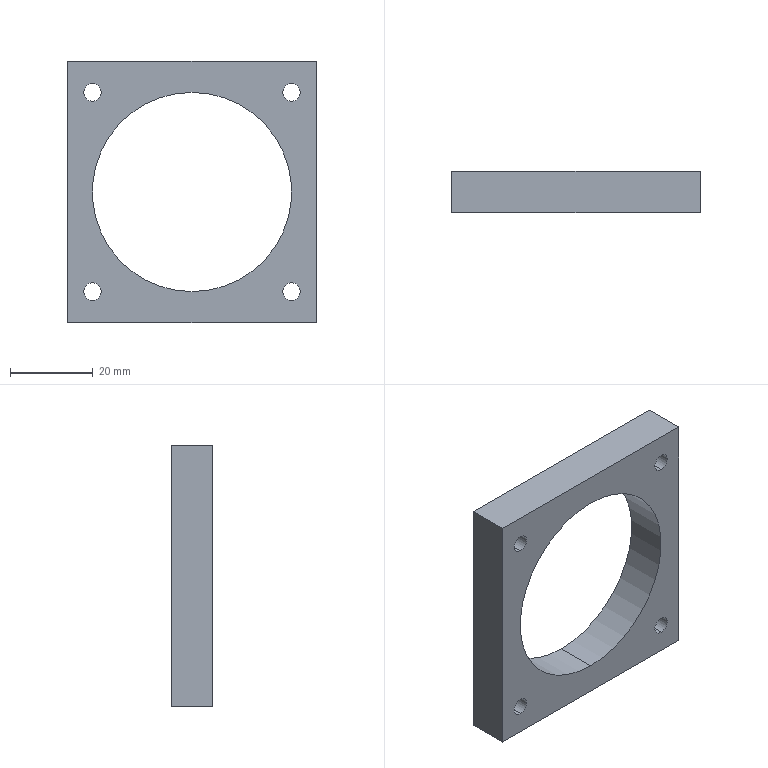Part | STEP file | 连接Plate 3 | 1 solid | 16 faces | box 60 x 10 x 63 mm | volume 19150 mm3 | cylinder 10 | plane 6 | commonest cylinder face diameters 4.2 x8 48 x2
STEP:
#1=CARTESIAN_POINT('',(0.,0.,0.));
#2=DIRECTION('',(0.,0.,1.));
#3=DIRECTION('',(1.,0.,0.));
#4=AXIS2_PLACEMENT_3D('',#1,#2,#3);
#5=CARTESIAN_POINT('',(24.,10.,21.9));
#6=VERTEX_POINT('',#5);
#7=CARTESIAN_POINT('',(24.,0.,21.9));
#8=VERTEX_POINT('',#7);
#9=CARTESIAN_POINT('',(24.,0.,21.9));
#10=DIRECTION('',(0.,-1.,0.));
#11=VECTOR('',#10,1.);
#12=LINE('',#9,#11);
#13=CARTESIAN_POINT('',(24.,0.,24.));
#14=DIRECTION('',(0.,-1.,0.));
#15=DIRECTION('',(0.,0.,-1.));
#16=AXIS2_PLACEMENT_3D('',#13,#14,#15);
#17=CYLINDRICAL_SURFACE('',#16,2.1);
#18=CARTESIAN_POINT('',(6.283,0.));
#19=DIRECTION('',(0.,1.));
#20=VECTOR('',#19,1.);
#21=LINE('',#18,#20);
#22=(GEOMETRIC_REPRESENTATION_CONTEXT(2)PARAMETRIC_REPRESENTATION_CONTEXT()REPRESENTATION_CONTEXT('',''));
#23=DEFINITIONAL_REPRESENTATION('',(#21),#22);
#24=PCURVE('',#17,#23);
#25=CARTESIAN_POINT('',(24.,0.,24.));
#26=DIRECTION('',(0.,-1.,0.));
#27=DIRECTION('',(0.,0.,-1.));
#28=AXIS2_PLACEMENT_3D('',#25,#26,#27);
#29=CYLINDRICAL_SURFACE('',#28,2.1);
#30=CARTESIAN_POINT('',(0.,0.));
#31=DIRECTION('',(0.,1.));
#32=VECTOR('',#31,1.);
#33=LINE('',#30,#32);
#34=(GEOMETRIC_REPRESENTATION_CONTEXT(2)PARAMETRIC_REPRESENTATION_CONTEXT()REPRESENTATION_CONTEXT('',''));
#35=DEFINITIONAL_REPRESENTATION('',(#33),#34);
#36=PCURVE('',#29,#35);
#37=SURFACE_CURVE('',#12,(#24,#36),.PCURVE_S1.);
#38=EDGE_CURVE('',#6,#8,#37,.T.);
#39=ORIENTED_EDGE('',*,*,#38,.T.);
#40=CARTESIAN_POINT('',(24.,0.,26.1));
#41=VERTEX_POINT('',#40);
#42=CARTESIAN_POINT('',(24.,0.,24.));
#43=DIRECTION('',(0.,-1.,0.));
#44=DIRECTION('',(0.,0.,-1.));
#45=AXIS2_PLACEMENT_3D('',#42,#43,#44);
#46=CIRCLE('',#45,2.1);
#47=CARTESIAN_POINT('',(0.,0.));
#48=DIRECTION('',(1.,0.));
#49=VECTOR('',#48,1.);
#50=LINE('',#47,#49);
#51=(GEOMETRIC_REPRESENTATION_CONTEXT(2)PARAMETRIC_REPRESENTATION_CONTEXT()REPRESENTATION_CONTEXT('',''));
#52=DEFINITIONAL_REPRESENTATION('',(#50),#51);
#53=PCURVE('',#17,#52);
#54=CARTESIAN_POINT('',(0.,0.,0.));
#55=DIRECTION('',(0.,-1.,0.));
#56=DIRECTION('',(0.,0.,-1.));
#57=AXIS2_PLACEMENT_3D('',#54,#55,#56);
#58=PLANE('',#57);
#59=CARTESIAN_POINT('',(-24.,24.));
#60=DIRECTION('',(1.,0.));
#61=AXIS2_PLACEMENT_2D('',#59,#60);
#62=CIRCLE('',#61,2.1);
#63=(GEOMETRIC_REPRESENTATION_CONTEXT(2)PARAMETRIC_REPRESENTATION_CONTEXT()REPRESENTATION_CONTEXT('',''));
#64=DEFINITIONAL_REPRESENTATION('',(#62),#63);
#65=PCURVE('',#58,#64);
#66=SURFACE_CURVE('',#46,(#53,#65),.PCURVE_S1.);
#67=EDGE_CURVE('',#41,#8,#66,.T.);
#68=ORIENTED_EDGE('',*,*,#67,.F.);
#69=CARTESIAN_POINT('',(24.,10.,26.1));
#70=VERTEX_POINT('',#69);
#71=CARTESIAN_POINT('',(24.,0.,26.1));
#72=DIRECTION('',(0.,-1.,0.));
#73=VECTOR('',#72,1.);
#74=LINE('',#71,#73);
#75=CARTESIAN_POINT('',(3.142,0.));
#76=DIRECTION('',(0.,1.));
#77=VECTOR('',#76,1.);
#78=LINE('',#75,#77);
#79=(GEOMETRIC_REPRESENTATION_CONTEXT(2)PARAMETRIC_REPRESENTATION_CONTEXT()REPRESENTATION_CONTEXT('',''));
#80=DEFINITIONAL_REPRESENTATION('',(#78),#79);
#81=PCURVE('',#17,#80);
#82=CARTESIAN_POINT('',(3.142,0.));
#83=DIRECTION('',(0.,1.));
#84=VECTOR('',#83,1.);
#85=LINE('',#82,#84);
#86=(GEOMETRIC_REPRESENTATION_CONTEXT(2)PARAMETRIC_REPRESENTATION_CONTEXT()REPRESENTATION_CONTEXT('',''));
#87=DEFINITIONAL_REPRESENTATION('',(#85),#86);
#88=PCURVE('',#29,#87);
#89=SURFACE_CURVE('',#74,(#81,#88),.PCURVE_S1.);
#90=EDGE_CURVE('',#70,#41,#89,.T.);
#91=ORIENTED_EDGE('',*,*,#90,.F.);
#92=CARTESIAN_POINT('',(24.,10.,24.));
#93=DIRECTION('',(0.,-1.,0.));
#94=DIRECTION('',(0.,0.,-1.));
#95=AXIS2_PLACEMENT_3D('',#92,#93,#94);
#96=CIRCLE('',#95,2.1);
#97=CARTESIAN_POINT('',(0.,-10.));
#98=DIRECTION('',(1.,0.));
#99=VECTOR('',#98,1.);
#100=LINE('',#97,#99);
#101=(GEOMETRIC_REPRESENTATION_CONTEXT(2)PARAMETRIC_REPRESENTATION_CONTEXT()REPRESENTATION_CONTEXT('',''));
#102=DEFINITIONAL_REPRESENTATION('',(#100),#101);
#103=PCURVE('',#17,#102);
#104=CARTESIAN_POINT('',(0.,10.,0.));
#105=DIRECTION('',(0.,-1.,0.));
#106=DIRECTION('',(0.,0.,-1.));
#107=AXIS2_PLACEMENT_3D('',#104,#105,#106);
#108=PLANE('',#107);
#109=CARTESIAN_POINT('',(-24.,24.));
#110=DIRECTION('',(1.,0.));
#111=AXIS2_PLACEMENT_2D('',#109,#110);
#112=CIRCLE('',#111,2.1);
#113=(GEOMETRIC_REPRESENTATION_CONTEXT(2)PARAMETRIC_REPRESENTATION_CONTEXT()REPRESENTATION_CONTEXT('',''));
#114=DEFINITIONAL_REPRESENTATION('',(#112),#113);
#115=PCURVE('',#108,#114);
#116=SURFACE_CURVE('',#96,(#103,#115),.PCURVE_S1.);
#117=EDGE_CURVE('',#70,#6,#116,.T.);
#118=ORIENTED_EDGE('',*,*,#117,.T.);
#119=EDGE_LOOP('',(#39,#68,#91,#118));
#120=FACE_BOUND('',#119,.F.);
#121=ADVANCED_FACE('',(#120),#17,.F.);
#122=CARTESIAN_POINT('',(24.,10.,-26.1));
#123=VERTEX_POINT('',#122);
#124=CARTESIAN_POINT('',(24.,0.,-26.1));
#125=VERTEX_POINT('',#124);
#126=CARTESIAN_POINT('',(24.,0.,-26.1));
#127=DIRECTION('',(0.,-1.,0.));
#128=VECTOR('',#127,1.);
#129=LINE('',#126,#128);
#130=CARTESIAN_POINT('',(24.,0.,-24.));
#131=DIRECTION('',(0.,-1.,0.));
#132=DIRECTION('',(0.,0.,-1.));
#133=AXIS2_PLACEMENT_3D('',#130,#131,#132);
#134=CYLINDRICAL_SURFACE('',#133,2.1);
#135=CARTESIAN_POINT('',(6.283,0.));
#136=DIRECTION('',(0.,1.));
#137=VECTOR('',#136,1.);
#138=LINE('',#135,#137);
#139=(GEOMETRIC_REPRESENTATION_CONTEXT(2)PARAMETRIC_REPRESENTATION_CONTEXT()REPRESENTATION_CONTEXT('',''));
#140=DEFINITIONAL_REPRESENTATION('',(#138),#139);
#141=PCURVE('',#134,#140);
#142=CARTESIAN_POINT('',(24.,0.,-24.));
#143=DIRECTION('',(0.,-1.,0.));
#144=DIRECTION('',(0.,0.,-1.));
#145=AXIS2_PLACEMENT_3D('',#142,#143,#144);
#146=CYLINDRICAL_SURFACE('',#145,2.1);
#147=CARTESIAN_POINT('',(0.,0.));
#148=DIRECTION('',(0.,1.));
#149=VECTOR('',#148,1.);
#150=LINE('',#147,#149);
#151=(GEOMETRIC_REPRESENTATION_CONTEXT(2)PARAMETRIC_REPRESENTATION_CONTEXT()REPRESENTATION_CONTEXT('',''));
#152=DEFINITIONAL_REPRESENTATION('',(#150),#151);
#153=PCURVE('',#146,#152);
#154=SURFACE_CURVE('',#129,(#141,#153),.PCURVE_S1.);
#155=EDGE_CURVE('',#123,#125,#154,.T.);
#156=ORIENTED_EDGE('',*,*,#155,.T.);
#157=CARTESIAN_POINT('',(24.,0.,-21.9));
#158=VERTEX_POINT('',#157);
#159=CARTESIAN_POINT('',(24.,0.,-24.));
#160=DIRECTION('',(0.,-1.,0.));
#161=DIRECTION('',(0.,0.,-1.));
#162=AXIS2_PLACEMENT_3D('',#159,#160,#161);
#163=CIRCLE('',#162,2.1);
#164=CARTESIAN_POINT('',(0.,0.));
#165=DIRECTION('',(1.,0.));
#166=VECTOR('',#165,1.);
#167=LINE('',#164,#166);
#168=(GEOMETRIC_REPRESENTATION_CONTEXT(2)PARAMETRIC_REPRESENTATION_CONTEXT()REPRESENTATION_CONTEXT('',''));
#169=DEFINITIONAL_REPRESENTATION('',(#167),#168);
#170=PCURVE('',#134,#169);
#171=CARTESIAN_POINT('',(24.,24.));
#172=DIRECTION('',(1.,0.));
#173=AXIS2_PLACEMENT_2D('',#171,#172);
#174=CIRCLE('',#173,2.1);
#175=(GEOMETRIC_REPRESENTATION_CONTEXT(2)PARAMETRIC_REPRESENTATION_CONTEXT()REPRESENTATION_CONTEXT('',''));
#176=DEFINITIONAL_REPRESENTATION('',(#174),#175);
#177=PCURVE('',#58,#176);
#178=SURFACE_CURVE('',#163,(#170,#177),.PCURVE_S1.);
#179=EDGE_CURVE('',#158,#125,#178,.T.);
#180=ORIENTED_EDGE('',*,*,#179,.F.);
#181=CARTESIAN_POINT('',(24.,10.,-21.9));
#182=VERTEX_POINT('',#181);
#183=CARTESIAN_POINT('',(24.,0.,-21.9));
#184=DIRECTION('',(0.,-1.,0.));
#185=VECTOR('',#184,1.);
#186=LINE('',#183,#185);
#187=CARTESIAN_POINT('',(3.142,0.));
#188=DIRECTION('',(0.,1.));
#189=VECTOR('',#188,1.);
#190=LINE('',#187,#189);
#191=(GEOMETRIC_REPRESENTATION_CONTEXT(2)PARAMETRIC_REPRESENTATION_CONTEXT()REPRESENTATION_CONTEXT('',''));
#192=DEFINITIONAL_REPRESENTATION('',(#190),#191);
#193=PCURVE('',#134,#192);
#194=CARTESIAN_POINT('',(3.142,0.));
#195=DIRECTION('',(0.,1.));
#196=VECTOR('',#195,1.);
#197=LINE('',#194,#196);
#198=(GEOMETRIC_REPRESENTATION_CONTEXT(2)PARAMETRIC_REPRESENTATION_CONTEXT()REPRESENTATION_CONTEXT('',''));
#199=DEFINITIONAL_REPRESENTATION('',(#197),#198);
#200=PCURVE('',#146,#199);
#201=SURFACE_CURVE('',#186,(#193,#200),.PCURVE_S1.);
#202=EDGE_CURVE('',#182,#158,#201,.T.);
#203=ORIENTED_EDGE('',*,*,#202,.F.);
#204=CARTESIAN_POINT('',(24.,10.,-24.));
#205=DIRECTION('',(0.,-1.,0.));
#206=DIRECTION('',(0.,0.,-1.));
#207=AXIS2_PLACEMENT_3D('',#204,#205,#206);
#208=CIRCLE('',#207,2.1);
#209=CARTESIAN_POINT('',(0.,-10.));
#210=DIRECTION('',(1.,0.));
#211=VECTOR('',#210,1.);
#212=LINE('',#209,#211);
#213=(GEOMETRIC_REPRESENTATION_CONTEXT(2)PARAMETRIC_REPRESENTATION_CONTEXT()REPRESENTATION_CONTEXT('',''));
#214=DEFINITIONAL_REPRESENTATION('',(#212),#213);
#215=PCURVE('',#134,#214);
#216=CARTESIAN_POINT('',(24.,24.));
#217=DIRECTION('',(1.,0.));
#218=AXIS2_PLACEMENT_2D('',#216,#217);
#219=CIRCLE('',#218,2.1);
#220=(GEOMETRIC_REPRESENTATION_CONTEXT(2)PARAMETRIC_REPRESENTATION_CONTEXT()REPRESENTATION_CONTEXT('',''));
#221=DEFINITIONAL_REPRESENTATION('',(#219),#220);
#222=PCURVE('',#108,#221);
#223=SURFACE_CURVE('',#208,(#215,#222),.PCURVE_S1.);
#224=EDGE_CURVE('',#182,#123,#223,.T.);
#225=ORIENTED_EDGE('',*,*,#224,.T.);
#226=EDGE_LOOP('',(#156,#180,#203,#225));
#227=FACE_BOUND('',#226,.F.);
#228=ADVANCED_FACE('',(#227),#134,.F.);
#229=CARTESIAN_POINT('',(-24.,10.,21.9));
#230=VERTEX_POINT('',#229);
#231=CARTESIAN_POINT('',(-24.,0.,21.9));
#232=VERTEX_POINT('',#231);
#233=CARTESIAN_POINT('',(-24.,0.,21.9));
#234=DIRECTION('',(0.,-1.,0.));
#235=VECTOR('',#234,1.);
#236=LINE('',#233,#235);
#237=CARTESIAN_POINT('',(-24.,0.,24.));
#238=DIRECTION('',(0.,-1.,0.));
#239=DIRECTION('',(0.,0.,-1.));
#240=AXIS2_PLACEMENT_3D('',#237,#238,#239);
#241=CYLINDRICAL_SURFACE('',#240,2.1);
#242=CARTESIAN_POINT('',(6.283,0.));
#243=DIRECTION('',(0.,1.));
#244=VECTOR('',#243,1.);
#245=LINE('',#242,#244);
#246=(GEOMETRIC_REPRESENTATION_CONTEXT(2)PARAMETRIC_REPRESENTATION_CONTEXT()REPRESENTATION_CONTEXT('',''));
#247=DEFINITIONAL_REPRESENTATION('',(#245),#246);
#248=PCURVE('',#241,#247);
#249=CARTESIAN_POINT('',(-24.,0.,24.));
#250=DIRECTION('',(0.,-1.,0.));
#251=DIRECTION('',(0.,0.,-1.));
#252=AXIS2_PLACEMENT_3D('',#249,#250,#251);
#253=CYLINDRICAL_SURFACE('',#252,2.1);
#254=CARTESIAN_POINT('',(0.,0.));
#255=DIRECTION('',(0.,1.));
#256=VECTOR('',#255,1.);
#257=LINE('',#254,#256);
#258=(GEOMETRIC_REPRESENTATION_CONTEXT(2)PARAMETRIC_REPRESENTATION_CONTEXT()REPRESENTATION_CONTEXT('',''));
#259=DEFINITIONAL_REPRESENTATION('',(#257),#258);
#260=PCURVE('',#253,#259);
#261=SURFACE_CURVE('',#236,(#248,#260),.PCURVE_S1.);
#262=EDGE_CURVE('',#230,#232,#261,.T.);
#263=ORIENTED_EDGE('',*,*,#262,.T.);
#264=CARTESIAN_POINT('',(-24.,0.,26.1));
#265=VERTEX_POINT('',#264);
#266=CARTESIAN_POINT('',(-24.,0.,24.));
#267=DIRECTION('',(0.,-1.,0.));
#268=DIRECTION('',(0.,0.,-1.));
#269=AXIS2_PLACEMENT_3D('',#266,#267,#268);
#270=CIRCLE('',#269,2.1);
#271=CARTESIAN_POINT('',(0.,0.));
#272=DIRECTION('',(1.,0.));
#273=VECTOR('',#272,1.);
#274=LINE('',#271,#273);
#275=(GEOMETRIC_REPRESENTATION_CONTEXT(2)PARAMETRIC_REPRESENTATION_CONTEXT()REPRESENTATION_CONTEXT('',''));
#276=DEFINITIONAL_REPRESENTATION('',(#274),#275);
#277=PCURVE('',#241,#276);
#278=CARTESIAN_POINT('',(-24.,-24.));
#279=DIRECTION('',(1.,0.));
#280=AXIS2_PLACEMENT_2D('',#278,#279);
#281=CIRCLE('',#280,2.1);
#282=(GEOMETRIC_REPRESENTATION_CONTEXT(2)PARAMETRIC_REPRESENTATION_CONTEXT()REPRESENTATION_CONTEXT('',''));
#283=DEFINITIONAL_REPRESENTATION('',(#281),#282);
#284=PCURVE('',#58,#283);
#285=SURFACE_CURVE('',#270,(#277,#284),.PCURVE_S1.);
#286=EDGE_CURVE('',#265,#232,#285,.T.);
#287=ORIENTED_EDGE('',*,*,#286,.F.);
#288=CARTESIAN_POINT('',(-24.,10.,26.1));
#289=VERTEX_POINT('',#288);
#290=CARTESIAN_POINT('',(-24.,0.,26.1));
#291=DIRECTION('',(0.,-1.,0.));
#292=VECTOR('',#291,1.);
#293=LINE('',#290,#292);
#294=CARTESIAN_POINT('',(3.142,0.));
#295=DIRECTION('',(0.,1.));
#296=VECTOR('',#295,1.);
#297=LINE('',#294,#296);
#298=(GEOMETRIC_REPRESENTATION_CONTEXT(2)PARAMETRIC_REPRESENTATION_CONTEXT()REPRESENTATION_CONTEXT('',''));
#299=DEFINITIONAL_REPRESENTATION('',(#297),#298);
#300=PCURVE('',#241,#299);
#301=CARTESIAN_POINT('',(3.142,0.));
#302=DIRECTION('',(0.,1.));
#303=VECTOR('',#302,1.);
#304=LINE('',#301,#303);
#305=(GEOMETRIC_REPRESENTATION_CONTEXT(2)PARAMETRIC_REPRESENTATION_CONTEXT()REPRESENTATION_CONTEXT('',''));
#306=DEFINITIONAL_REPRESENTATION('',(#304),#305);
#307=PCURVE('',#253,#306);
#308=SURFACE_CURVE('',#293,(#300,#307),.PCURVE_S1.);
#309=EDGE_CURVE('',#289,#265,#308,.T.);
#310=ORIENTED_EDGE('',*,*,#309,.F.);
#311=CARTESIAN_POINT('',(-24.,10.,24.));
#312=DIRECTION('',(0.,-1.,0.));
#313=DIRECTION('',(0.,0.,-1.));
#314=AXIS2_PLACEMENT_3D('',#311,#312,#313);
#315=CIRCLE('',#314,2.1);
#316=CARTESIAN_POINT('',(0.,-10.));
#317=DIRECTION('',(1.,0.));
#318=VECTOR('',#317,1.);
#319=LINE('',#316,#318);
#320=(GEOMETRIC_REPRESENTATION_CONTEXT(2)PARAMETRIC_REPRESENTATION_CONTEXT()REPRESENTATION_CONTEXT('',''));
#321=DEFINITIONAL_REPRESENTATION('',(#319),#320);
#322=PCURVE('',#241,#321);
#323=CARTESIAN_POINT('',(-24.,-24.));
#324=DIRECTION('',(1.,0.));
#325=AXIS2_PLACEMENT_2D('',#323,#324);
#326=CIRCLE('',#325,2.1);
#327=(GEOMETRIC_REPRESENTATION_CONTEXT(2)PARAMETRIC_REPRESENTATION_CONTEXT()REPRESENTATION_CONTEXT('',''));
#328=DEFINITIONAL_REPRESENTATION('',(#326),#327);
#329=PCURVE('',#108,#328);
#330=SURFACE_CURVE('',#315,(#322,#329),.PCURVE_S1.);
#331=EDGE_CURVE('',#289,#230,#330,.T.);
#332=ORIENTED_EDGE('',*,*,#331,.T.);
#333=EDGE_LOOP('',(#263,#287,#310,#332));
#334=FACE_BOUND('',#333,.F.);
#335=ADVANCED_FACE('',(#334),#241,.F.);
#336=CARTESIAN_POINT('',(-24.,10.,-26.1));
#337=VERTEX_POINT('',#336);
#338=CARTESIAN_POINT('',(-24.,0.,-26.1));
#339=VERTEX_POINT('',#338);
#340=CARTESIAN_POINT('',(-24.,0.,-26.1));
#341=DIRECTION('',(0.,-1.,0.));
#342=VECTOR('',#341,1.);
#343=LINE('',#340,#342);
#344=CARTESIAN_POINT('',(-24.,0.,-24.));
#345=DIRECTION('',(0.,-1.,0.));
#346=DIRECTION('',(0.,0.,-1.));
#347=AXIS2_PLACEMENT_3D('',#344,#345,#346);
#348=CYLINDRICAL_SURFACE('',#347,2.1);
#349=CARTESIAN_POINT('',(6.283,0.));
#350=DIRECTION('',(0.,1.));
#351=VECTOR('',#350,1.);
#352=LINE('',#349,#351);
#353=(GEOMETRIC_REPRESENTATION_CONTEXT(2)PARAMETRIC_REPRESENTATION_CONTEXT()REPRESENTATION_CONTEXT('',''));
#354=DEFINITIONAL_REPRESENTATION('',(#352),#353);
#355=PCURVE('',#348,#354);
#356=CARTESIAN_POINT('',(-24.,0.,-24.));
#357=DIRECTION('',(0.,-1.,0.));
#358=DIRECTION('',(0.,0.,-1.));
#359=AXIS2_PLACEMENT_3D('',#356,#357,#358);
#360=CYLINDRICAL_SURFACE('',#359,2.1);
#361=CARTESIAN_POINT('',(0.,0.));
#362=DIRECTION('',(0.,1.));
#363=VECTOR('',#362,1.);
#364=LINE('',#361,#363);
#365=(GEOMETRIC_REPRESENTATION_CONTEXT(2)PARAMETRIC_REPRESENTATION_CONTEXT()REPRESENTATION_CONTEXT('',''));
#366=DEFINITIONAL_REPRESENTATION('',(#364),#365);
#367=PCURVE('',#360,#366);
#368=SURFACE_CURVE('',#343,(#355,#367),.PCURVE_S1.);
#369=EDGE_CURVE('',#337,#339,#368,.T.);
#370=ORIENTED_EDGE('',*,*,#369,.T.);
#371=CARTESIAN_POINT('',(-24.,0.,-21.9));
#372=VERTEX_POINT('',#371);
#373=CARTESIAN_POINT('',(-24.,0.,-24.));
#374=DIRECTION('',(0.,-1.,0.));
#375=DIRECTION('',(0.,0.,-1.));
#376=AXIS2_PLACEMENT_3D('',#373,#374,#375);
#377=CIRCLE('',#376,2.1);
#378=CARTESIAN_POINT('',(0.,0.));
#379=DIRECTION('',(1.,0.));
#380=VECTOR('',#379,1.);
#381=LINE('',#378,#380);
#382=(GEOMETRIC_REPRESENTATION_CONTEXT(2)PARAMETRIC_REPRESENTATION_CONTEXT()REPRESENTATION_CONTEXT('',''));
#383=DEFINITIONAL_REPRESENTATION('',(#381),#382);
#384=PCURVE('',#348,#383);
#385=CARTESIAN_POINT('',(24.,-24.));
#386=DIRECTION('',(1.,0.));
#387=AXIS2_PLACEMENT_2D('',#385,#386);
#388=CIRCLE('',#387,2.1);
#389=(GEOMETRIC_REPRESENTATION_CONTEXT(2)PARAMETRIC_REPRESENTATION_CONTEXT()REPRESENTATION_CONTEXT('',''));
#390=DEFINITIONAL_REPRESENTATION('',(#388),#389);
#391=PCURVE('',#58,#390);
#392=SURFACE_CURVE('',#377,(#384,#391),.PCURVE_S1.);
#393=EDGE_CURVE('',#372,#339,#392,.T.);
#394=ORIENTED_EDGE('',*,*,#393,.F.);
#395=CARTESIAN_POINT('',(-24.,10.,-21.9));
#396=VERTEX_POINT('',#395);
#397=CARTESIAN_POINT('',(-24.,0.,-21.9));
#398=DIRECTION('',(0.,-1.,0.));
#399=VECTOR('',#398,1.);
#400=LINE('',#397,#399);
#401=CARTESIAN_POINT('',(3.142,0.));
#402=DIRECTION('',(0.,1.));
#403=VECTOR('',#402,1.);
#404=LINE('',#401,#403);
#405=(GEOMETRIC_REPRESENTATION_CONTEXT(2)PARAMETRIC_REPRESENTATION_CONTEXT()REPRESENTATION_CONTEXT('',''));
#406=DEFINITIONAL_REPRESENTATION('',(#404),#405);
#407=PCURVE('',#348,#406);
#408=CARTESIAN_POINT('',(3.142,0.));
#409=DIRECTION('',(0.,1.));
#410=VECTOR('',#409,1.);
#411=LINE('',#408,#410);
#412=(GEOMETRIC_REPRESENTATION_CONTEXT(2)PARAMETRIC_REPRESENTATION_CONTEXT()REPRESENTATION_CONTEXT('',''));
#413=DEFINITIONAL_REPRESENTATION('',(#411),#412);
#414=PCURVE('',#360,#413);
#415=SURFACE_CURVE('',#400,(#407,#414),.PCURVE_S1.);
#416=EDGE_CURVE('',#396,#372,#415,.T.);
#417=ORIENTED_EDGE('',*,*,#416,.F.);
#418=CARTESIAN_POINT('',(-24.,10.,-24.));
#419=DIRECTION('',(0.,-1.,0.));
#420=DIRECTION('',(0.,0.,-1.));
#421=AXIS2_PLACEMENT_3D('',#418,#419,#420);
#422=CIRCLE('',#421,2.1);
#423=CARTESIAN_POINT('',(0.,-10.));
#424=DIRECTION('',(1.,0.));
#425=VECTOR('',#424,1.);
#426=LINE('',#423,#425);
#427=(GEOMETRIC_REPRESENTATION_CONTEXT(2)PARAMETRIC_REPRESENTATION_CONTEXT()REPRESENTATION_CONTEXT('',''));
#428=DEFINITIONAL_REPRESENTATION('',(#426),#427);
#429=PCURVE('',#348,#428);
#430=CARTESIAN_POINT('',(24.,-24.));
#431=DIRECTION('',(1.,0.));
#432=AXIS2_PLACEMENT_2D('',#430,#431);
#433=CIRCLE('',#432,2.1);
#434=(GEOMETRIC_REPRESENTATION_CONTEXT(2)PARAMETRIC_REPRESENTATION_CONTEXT()REPRESENTATION_CONTEXT('',''));
#435=DEFINITIONAL_REPRESENTATION('',(#433),#434);
#436=PCURVE('',#108,#435);
#437=SURFACE_CURVE('',#422,(#429,#436),.PCURVE_S1.);
#438=EDGE_CURVE('',#396,#337,#437,.T.);
#439=ORIENTED_EDGE('',*,*,#438,.T.);
#440=EDGE_LOOP('',(#370,#394,#417,#439));
#441=FACE_BOUND('',#440,.F.);
#442=ADVANCED_FACE('',(#441),#348,.F.);
#443=CARTESIAN_POINT('',(0.,0.,24.));
#444=VERTEX_POINT('',#443);
#445=CARTESIAN_POINT('',(0.,10.,24.));
#446=VERTEX_POINT('',#445);
#447=CARTESIAN_POINT('',(0.,0.,24.));
#448=DIRECTION('',(0.,1.,0.));
#449=VECTOR('',#448,1.);
#450=LINE('',#447,#449);
#451=CARTESIAN_POINT('',(0.,0.,0.));
#452=DIRECTION('',(0.,1.,0.));
#453=DIRECTION('',(0.,0.,1.));
#454=AXIS2_PLACEMENT_3D('',#451,#452,#453);
#455=CYLINDRICAL_SURFACE('',#454,24.);
#456=CARTESIAN_POINT('',(6.283,0.));
#457=DIRECTION('',(0.,1.));
#458=VECTOR('',#457,1.);
#459=LINE('',#456,#458);
#460=(GEOMETRIC_REPRESENTATION_CONTEXT(2)PARAMETRIC_REPRESENTATION_CONTEXT()REPRESENTATION_CONTEXT('',''));
#461=DEFINITIONAL_REPRESENTATION('',(#459),#460);
#462=PCURVE('',#455,#461);
#463=CARTESIAN_POINT('',(0.,0.,0.));
#464=DIRECTION('',(0.,1.,0.));
#465=DIRECTION('',(0.,0.,1.));
#466=AXIS2_PLACEMENT_3D('',#463,#464,#465);
#467=CYLINDRICAL_SURFACE('',#466,24.);
#468=CARTESIAN_POINT('',(0.,0.));
#469=DIRECTION('',(0.,1.));
#470=VECTOR('',#469,1.);
#471=LINE('',#468,#470);
#472=(GEOMETRIC_REPRESENTATION_CONTEXT(2)PARAMETRIC_REPRESENTATION_CONTEXT()REPRESENTATION_CONTEXT('',''));
#473=DEFINITIONAL_REPRESENTATION('',(#471),#472);
#474=PCURVE('',#467,#473);
#475=SURFACE_CURVE('',#450,(#462,#474),.PCURVE_S1.);
#476=EDGE_CURVE('',#444,#446,#475,.T.);
#477=ORIENTED_EDGE('',*,*,#476,.T.);
#478=CARTESIAN_POINT('',(0.,10.,-24.));
#479=VERTEX_POINT('',#478);
#480=CARTESIAN_POINT('',(0.,10.,0.));
#481=DIRECTION('',(0.,1.,0.));
#482=DIRECTION('',(0.,0.,1.));
#483=AXIS2_PLACEMENT_3D('',#480,#481,#482);
#484=CIRCLE('',#483,24.);
#485=CARTESIAN_POINT('',(0.,10.));
#486=DIRECTION('',(1.,0.));
#487=VECTOR('',#486,1.);
#488=LINE('',#485,#487);
#489=(GEOMETRIC_REPRESENTATION_CONTEXT(2)PARAMETRIC_REPRESENTATION_CONTEXT()REPRESENTATION_CONTEXT('',''));
#490=DEFINITIONAL_REPRESENTATION('',(#488),#489);
#491=PCURVE('',#455,#490);
#492=CARTESIAN_POINT('',(-24.,0.));
#493=CARTESIAN_POINT('',(-24.,41.569));
#494=CARTESIAN_POINT('',(12.,20.785));
#495=CARTESIAN_POINT('',(48.,0.));
#496=CARTESIAN_POINT('',(12.,-20.785));
#497=CARTESIAN_POINT('',(-24.,-41.569));
#498=CARTESIAN_POINT('',(-24.,0.));
#499=(BOUNDED_CURVE()B_SPLINE_CURVE(2,(#492,#493,#494,#495,#496,#497,#498),.UNSPECIFIED.,.T.,.F.)B_SPLINE_CURVE_WITH_KNOTS((1,2,2,2,2,1),(-2.094,0.,2.094,4.189,6.283,8.378),.UNSPECIFIED.)CURVE()GEOMETRIC_REPRESENTATION_ITEM()RATIONAL_B_SPLINE_CURVE((1.,0.5,1.,0.5,1.,0.5,1.))REPRESENTATION_ITEM(''));
#500=(GEOMETRIC_REPRESENTATION_CONTEXT(2)PARAMETRIC_REPRESENTATION_CONTEXT()REPRESENTATION_CONTEXT('',''));
#501=DEFINITIONAL_REPRESENTATION('',(#499),#500);
#502=PCURVE('',#108,#501);
#503=SURFACE_CURVE('',#484,(#491,#502),.PCURVE_S1.);
#504=EDGE_CURVE('',#479,#446,#503,.T.);
#505=ORIENTED_EDGE('',*,*,#504,.F.);
#506=CARTESIAN_POINT('',(0.,0.,-24.));
#507=VERTEX_POINT('',#506);
#508=CARTESIAN_POINT('',(0.,0.,-24.));
#509=DIRECTION('',(0.,1.,0.));
#510=VECTOR('',#509,1.);
#511=LINE('',#508,#510);
#512=CARTESIAN_POINT('',(3.142,0.));
#513=DIRECTION('',(0.,1.));
#514=VECTOR('',#513,1.);
#515=LINE('',#512,#514);
#516=(GEOMETRIC_REPRESENTATION_CONTEXT(2)PARAMETRIC_REPRESENTATION_CONTEXT()REPRESENTATION_CONTEXT('',''));
#517=DEFINITIONAL_REPRESENTATION('',(#515),#516);
#518=PCURVE('',#455,#517);
#519=CARTESIAN_POINT('',(3.142,0.));
#520=DIRECTION('',(0.,1.));
#521=VECTOR('',#520,1.);
#522=LINE('',#519,#521);
#523=(GEOMETRIC_REPRESENTATION_CONTEXT(2)PARAMETRIC_REPRESENTATION_CONTEXT()REPRESENTATION_CONTEXT('',''));
#524=DEFINITIONAL_REPRESENTATION('',(#522),#523);
#525=PCURVE('',#467,#524);
#526=SURFACE_CURVE('',#511,(#518,#525),.PCURVE_S1.);
#527=EDGE_CURVE('',#507,#479,#526,.T.);
#528=ORIENTED_EDGE('',*,*,#527,.F.);
#529=CARTESIAN_POINT('',(0.,0.,0.));
#530=DIRECTION('',(0.,1.,0.));
#531=DIRECTION('',(0.,0.,1.));
#532=AXIS2_PLACEMENT_3D('',#529,#530,#531);
#533=CIRCLE('',#532,24.);
#534=CARTESIAN_POINT('',(0.,0.));
#535=DIRECTION('',(1.,0.));
#536=VECTOR('',#535,1.);
#537=LINE('',#534,#536);
#538=(GEOMETRIC_REPRESENTATION_CONTEXT(2)PARAMETRIC_REPRESENTATION_CONTEXT()REPRESENTATION_CONTEXT('',''));
#539=DEFINITIONAL_REPRESENTATION('',(#537),#538);
#540=PCURVE('',#455,#539);
#541=CARTESIAN_POINT('',(-24.,0.));
#542=CARTESIAN_POINT('',(-24.,41.569));
#543=CARTESIAN_POINT('',(12.,20.785));
#544=CARTESIAN_POINT('',(48.,0.));
#545=CARTESIAN_POINT('',(12.,-20.785));
#546=CARTESIAN_POINT('',(-24.,-41.569));
#547=CARTESIAN_POINT('',(-24.,0.));
#548=(BOUNDED_CURVE()B_SPLINE_CURVE(2,(#541,#542,#543,#544,#545,#546,#547),.UNSPECIFIED.,.T.,.F.)B_SPLINE_CURVE_WITH_KNOTS((1,2,2,2,2,1),(-2.094,0.,2.094,4.189,6.283,8.378),.UNSPECIFIED.)CURVE()GEOMETRIC_REPRESENTATION_ITEM()RATIONAL_B_SPLINE_CURVE((1.,0.5,1.,0.5,1.,0.5,1.))REPRESENTATION_ITEM(''));
#549=(GEOMETRIC_REPRESENTATION_CONTEXT(2)PARAMETRIC_REPRESENTATION_CONTEXT()REPRESENTATION_CONTEXT('',''));
#550=DEFINITIONAL_REPRESENTATION('',(#548),#549);
#551=PCURVE('',#58,#550);
#552=SURFACE_CURVE('',#533,(#540,#551),.PCURVE_S1.);
#553=EDGE_CURVE('',#507,#444,#552,.T.);
#554=ORIENTED_EDGE('',*,*,#553,.T.);
#555=EDGE_LOOP('',(#477,#505,#528,#554));
#556=FACE_BOUND('',#555,.F.);
#557=ADVANCED_FACE('',(#556),#455,.F.);
#558=CARTESIAN_POINT('',(30.,0.,31.5));
#559=VERTEX_POINT('',#558);
#560=CARTESIAN_POINT('',(30.,0.,-31.5));
#561=VERTEX_POINT('',#560);
#562=CARTESIAN_POINT('',(30.,0.,31.5));
#563=DIRECTION('',(0.,0.,-1.));
#564=VECTOR('',#563,1.);
#565=LINE('',#562,#564);
#566=CARTESIAN_POINT('',(30.,10.,31.5));
#567=DIRECTION('',(-1.,0.,0.));
#568=DIRECTION('',(0.,0.,1.));
#569=AXIS2_PLACEMENT_3D('',#566,#567,#568);
#570=PLANE('',#569);
#571=CARTESIAN_POINT('',(0.,-10.));
#572=DIRECTION('',(-1.,0.));
#573=VECTOR('',#572,1.);
#574=LINE('',#571,#573);
#575=(GEOMETRIC_REPRESENTATION_CONTEXT(2)PARAMETRIC_REPRESENTATION_CONTEXT()REPRESENTATION_CONTEXT('',''));
#576=DEFINITIONAL_REPRESENTATION('',(#574),#575);
#577=PCURVE('',#570,#576);
#578=CARTESIAN_POINT('',(-31.5,30.));
#579=DIRECTION('',(1.,0.));
#580=VECTOR('',#579,1.);
#581=LINE('',#578,#580);
#582=(GEOMETRIC_REPRESENTATION_CONTEXT(2)PARAMETRIC_REPRESENTATION_CONTEXT()REPRESENTATION_CONTEXT('',''));
#583=DEFINITIONAL_REPRESENTATION('',(#581),#582);
#584=PCURVE('',#58,#583);
#585=SURFACE_CURVE('',#565,(#577,#584),.PCURVE_S1.);
#586=EDGE_CURVE('',#559,#561,#585,.T.);
#587=ORIENTED_EDGE('',*,*,#586,.T.);
#588=CARTESIAN_POINT('',(30.,10.,-31.5));
#589=VERTEX_POINT('',#588);
#590=CARTESIAN_POINT('',(30.,10.,-31.5));
#591=DIRECTION('',(0.,-1.,0.));
#592=VECTOR('',#591,1.);
#593=LINE('',#590,#592);
#594=CARTESIAN_POINT('',(-63.,0.));
#595=DIRECTION('',(0.,-1.));
#596=VECTOR('',#595,1.);
#597=LINE('',#594,#596);
#598=(GEOMETRIC_REPRESENTATION_CONTEXT(2)PARAMETRIC_REPRESENTATION_CONTEXT()REPRESENTATION_CONTEXT('',''));
#599=DEFINITIONAL_REPRESENTATION('',(#597),#598);
#600=PCURVE('',#570,#599);
#601=CARTESIAN_POINT('',(-30.,10.,-31.5));
#602=DIRECTION('',(0.,0.,1.));
#603=DIRECTION('',(1.,0.,0.));
#604=AXIS2_PLACEMENT_3D('',#601,#602,#603);
#605=PLANE('',#604);
#606=CARTESIAN_POINT('',(60.,0.));
#607=DIRECTION('',(0.,-1.));
#608=VECTOR('',#607,1.);
#609=LINE('',#606,#608);
#610=(GEOMETRIC_REPRESENTATION_CONTEXT(2)PARAMETRIC_REPRESENTATION_CONTEXT()REPRESENTATION_CONTEXT('',''));
#611=DEFINITIONAL_REPRESENTATION('',(#609),#610);
#612=PCURVE('',#605,#611);
#613=SURFACE_CURVE('',#593,(#600,#612),.PCURVE_S1.);
#614=EDGE_CURVE('',#589,#561,#613,.T.);
#615=ORIENTED_EDGE('',*,*,#614,.F.);
#616=CARTESIAN_POINT('',(30.,10.,31.5));
#617=VERTEX_POINT('',#616);
#618=CARTESIAN_POINT('',(30.,10.,31.5));
#619=DIRECTION('',(0.,0.,-1.));
#620=VECTOR('',#619,1.);
#621=LINE('',#618,#620);
#622=CARTESIAN_POINT('',(0.,0.));
#623=DIRECTION('',(-1.,0.));
#624=VECTOR('',#623,1.);
#625=LINE('',#622,#624);
#626=(GEOMETRIC_REPRESENTATION_CONTEXT(2)PARAMETRIC_REPRESENTATION_CONTEXT()REPRESENTATION_CONTEXT('',''));
#627=DEFINITIONAL_REPRESENTATION('',(#625),#626);
#628=PCURVE('',#570,#627);
#629=CARTESIAN_POINT('',(-31.5,30.));
#630=DIRECTION('',(1.,0.));
#631=VECTOR('',#630,1.);
#632=LINE('',#629,#631);
#633=(GEOMETRIC_REPRESENTATION_CONTEXT(2)PARAMETRIC_REPRESENTATION_CONTEXT()REPRESENTATION_CONTEXT('',''));
#634=DEFINITIONAL_REPRESENTATION('',(#632),#633);
#635=PCURVE('',#108,#634);
#636=SURFACE_CURVE('',#621,(#628,#635),.PCURVE_S1.);
#637=EDGE_CURVE('',#617,#589,#636,.T.);
#638=ORIENTED_EDGE('',*,*,#637,.F.);
#639=CARTESIAN_POINT('',(30.,10.,31.5));
#640=DIRECTION('',(0.,-1.,0.));
#641=VECTOR('',#640,1.);
#642=LINE('',#639,#641);
#643=CARTESIAN_POINT('',(0.,0.));
#644=DIRECTION('',(0.,-1.));
#645=VECTOR('',#644,1.);
#646=LINE('',#643,#645);
#647=(GEOMETRIC_REPRESENTATION_CONTEXT(2)PARAMETRIC_REPRESENTATION_CONTEXT()REPRESENTATION_CONTEXT('',''));
#648=DEFINITIONAL_REPRESENTATION('',(#646),#647);
#649=PCURVE('',#570,#648);
#650=CARTESIAN_POINT('',(-30.,10.,31.5));
#651=DIRECTION('',(0.,0.,-1.));
#652=DIRECTION('',(-1.,0.,0.));
#653=AXIS2_PLACEMENT_3D('',#650,#651,#652);
#654=PLANE('',#653);
#655=CARTESIAN_POINT('',(-60.,0.));
#656=DIRECTION('',(0.,-1.));
#657=VECTOR('',#656,1.);
#658=LINE('',#655,#657);
#659=(GEOMETRIC_REPRESENTATION_CONTEXT(2)PARAMETRIC_REPRESENTATION_CONTEXT()REPRESENTATION_CONTEXT('',''));
#660=DEFINITIONAL_REPRESENTATION('',(#658),#659);
#661=PCURVE('',#654,#660);
#662=SURFACE_CURVE('',#642,(#649,#661),.PCURVE_S1.);
#663=EDGE_CURVE('',#617,#559,#662,.T.);
#664=ORIENTED_EDGE('',*,*,#663,.T.);
#665=EDGE_LOOP('',(#587,#615,#638,#664));
#666=FACE_BOUND('',#665,.T.);
#667=ADVANCED_FACE('',(#666),#570,.F.);
#668=CARTESIAN_POINT('',(-30.,0.,-31.5));
#669=VERTEX_POINT('',#668);
#670=CARTESIAN_POINT('',(-30.,0.,-31.5));
#671=DIRECTION('',(-1.,0.,0.));
#672=VECTOR('',#671,1.);
#673=LINE('',#670,#672);
#674=CARTESIAN_POINT('',(0.,-10.));
#675=DIRECTION('',(-1.,0.));
#676=VECTOR('',#675,1.);
#677=LINE('',#674,#676);
#678=(GEOMETRIC_REPRESENTATION_CONTEXT(2)PARAMETRIC_REPRESENTATION_CONTEXT()REPRESENTATION_CONTEXT('',''));
#679=DEFINITIONAL_REPRESENTATION('',(#677),#678);
#680=PCURVE('',#605,#679);
#681=CARTESIAN_POINT('',(31.5,-30.));
#682=DIRECTION('',(0.,-1.));
#683=VECTOR('',#682,1.);
#684=LINE('',#681,#683);
#685=(GEOMETRIC_REPRESENTATION_CONTEXT(2)PARAMETRIC_REPRESENTATION_CONTEXT()REPRESENTATION_CONTEXT('',''));
#686=DEFINITIONAL_REPRESENTATION('',(#684),#685);
#687=PCURVE('',#58,#686);
#688=SURFACE_CURVE('',#673,(#680,#687),.PCURVE_S1.);
#689=EDGE_CURVE('',#561,#669,#688,.T.);
#690=ORIENTED_EDGE('',*,*,#689,.T.);
#691=CARTESIAN_POINT('',(-30.,10.,-31.5));
#692=VERTEX_POINT('',#691);
#693=CARTESIAN_POINT('',(-30.,10.,-31.5));
#694=DIRECTION('',(0.,-1.,0.));
#695=VECTOR('',#694,1.);
#696=LINE('',#693,#695);
#697=CARTESIAN_POINT('',(0.,0.));
#698=DIRECTION('',(0.,-1.));
#699=VECTOR('',#698,1.);
#700=LINE('',#697,#699);
#701=(GEOMETRIC_REPRESENTATION_CONTEXT(2)PARAMETRIC_REPRESENTATION_CONTEXT()REPRESENTATION_CONTEXT('',''));
#702=DEFINITIONAL_REPRESENTATION('',(#700),#701);
#703=PCURVE('',#605,#702);
#704=CARTESIAN_POINT('',(-30.,10.,31.5));
#705=DIRECTION('',(1.,0.,0.));
#706=DIRECTION('',(0.,0.,-1.));
#707=AXIS2_PLACEMENT_3D('',#704,#705,#706);
#708=PLANE('',#707);
#709=CARTESIAN_POINT('',(63.,0.));
#710=DIRECTION('',(0.,-1.));
#711=VECTOR('',#710,1.);
#712=LINE('',#709,#711);
#713=(GEOMETRIC_REPRESENTATION_CONTEXT(2)PARAMETRIC_REPRESENTATION_CONTEXT()REPRESENTATION_CONTEXT('',''));
#714=DEFINITIONAL_REPRESENTATION('',(#712),#713);
#715=PCURVE('',#708,#714);
#716=SURFACE_CURVE('',#696,(#703,#715),.PCURVE_S1.);
#717=EDGE_CURVE('',#692,#669,#716,.T.);
#718=ORIENTED_EDGE('',*,*,#717,.F.);
#719=CARTESIAN_POINT('',(-30.,10.,-31.5));
#720=DIRECTION('',(-1.,0.,0.));
#721=VECTOR('',#720,1.);
#722=LINE('',#719,#721);
#723=CARTESIAN_POINT('',(0.,0.));
#724=DIRECTION('',(-1.,0.));
#725=VECTOR('',#724,1.);
#726=LINE('',#723,#725);
#727=(GEOMETRIC_REPRESENTATION_CONTEXT(2)PARAMETRIC_REPRESENTATION_CONTEXT()REPRESENTATION_CONTEXT('',''));
#728=DEFINITIONAL_REPRESENTATION('',(#726),#727);
#729=PCURVE('',#605,#728);
#730=CARTESIAN_POINT('',(31.5,-30.));
#731=DIRECTION('',(0.,-1.));
#732=VECTOR('',#731,1.);
#733=LINE('',#730,#732);
#734=(GEOMETRIC_REPRESENTATION_CONTEXT(2)PARAMETRIC_REPRESENTATION_CONTEXT()REPRESENTATION_CONTEXT('',''));
#735=DEFINITIONAL_REPRESENTATION('',(#733),#734);
#736=PCURVE('',#108,#735);
#737=SURFACE_CURVE('',#722,(#729,#736),.PCURVE_S1.);
#738=EDGE_CURVE('',#589,#692,#737,.T.);
#739=ORIENTED_EDGE('',*,*,#738,.F.);
#740=ORIENTED_EDGE('',*,*,#614,.T.);
#741=EDGE_LOOP('',(#690,#718,#739,#740));
#742=FACE_BOUND('',#741,.T.);
#743=ADVANCED_FACE('',(#742),#605,.F.);
#744=CARTESIAN_POINT('',(-30.,0.,31.5));
#745=VERTEX_POINT('',#744);
#746=CARTESIAN_POINT('',(-30.,0.,31.5));
#747=DIRECTION('',(0.,0.,1.));
#748=VECTOR('',#747,1.);
#749=LINE('',#746,#748);
#750=CARTESIAN_POINT('',(0.,-10.));
#751=DIRECTION('',(-1.,0.));
#752=VECTOR('',#751,1.);
#753=LINE('',#750,#752);
#754=(GEOMETRIC_REPRESENTATION_CONTEXT(2)PARAMETRIC_REPRESENTATION_CONTEXT()REPRESENTATION_CONTEXT('',''));
#755=DEFINITIONAL_REPRESENTATION('',(#753),#754);
#756=PCURVE('',#708,#755);
#757=CARTESIAN_POINT('',(-31.5,-30.));
#758=DIRECTION('',(-1.,0.));
#759=VECTOR('',#758,1.);
#760=LINE('',#757,#759);
#761=(GEOMETRIC_REPRESENTATION_CONTEXT(2)PARAMETRIC_REPRESENTATION_CONTEXT()REPRESENTATION_CONTEXT('',''));
#762=DEFINITIONAL_REPRESENTATION('',(#760),#761);
#763=PCURVE('',#58,#762);
#764=SURFACE_CURVE('',#749,(#756,#763),.PCURVE_S1.);
#765=EDGE_CURVE('',#669,#745,#764,.T.);
#766=ORIENTED_EDGE('',*,*,#765,.T.);
#767=CARTESIAN_POINT('',(-30.,10.,31.5));
#768=VERTEX_POINT('',#767);
#769=CARTESIAN_POINT('',(-30.,10.,31.5));
#770=DIRECTION('',(0.,-1.,0.));
#771=VECTOR('',#770,1.);
#772=LINE('',#769,#771);
#773=CARTESIAN_POINT('',(0.,0.));
#774=DIRECTION('',(0.,-1.));
#775=VECTOR('',#774,1.);
#776=LINE('',#773,#775);
#777=(GEOMETRIC_REPRESENTATION_CONTEXT(2)PARAMETRIC_REPRESENTATION_CONTEXT()REPRESENTATION_CONTEXT('',''));
#778=DEFINITIONAL_REPRESENTATION('',(#776),#777);
#779=PCURVE('',#708,#778);
#780=CARTESIAN_POINT('',(0.,0.));
#781=DIRECTION('',(0.,-1.));
#782=VECTOR('',#781,1.);
#783=LINE('',#780,#782);
#784=(GEOMETRIC_REPRESENTATION_CONTEXT(2)PARAMETRIC_REPRESENTATION_CONTEXT()REPRESENTATION_CONTEXT('',''));
#785=DEFINITIONAL_REPRESENTATION('',(#783),#784);
#786=PCURVE('',#654,#785);
#787=SURFACE_CURVE('',#772,(#779,#786),.PCURVE_S1.);
#788=EDGE_CURVE('',#768,#745,#787,.T.);
#789=ORIENTED_EDGE('',*,*,#788,.F.);
#790=CARTESIAN_POINT('',(-30.,10.,31.5));
#791=DIRECTION('',(0.,0.,1.));
#792=VECTOR('',#791,1.);
#793=LINE('',#790,#792);
#794=CARTESIAN_POINT('',(0.,0.));
#795=DIRECTION('',(-1.,0.));
#796=VECTOR('',#795,1.);
#797=LINE('',#794,#796);
#798=(GEOMETRIC_REPRESENTATION_CONTEXT(2)PARAMETRIC_REPRESENTATION_CONTEXT()REPRESENTATION_CONTEXT('',''));
#799=DEFINITIONAL_REPRESENTATION('',(#797),#798);
#800=PCURVE('',#708,#799);
#801=CARTESIAN_POINT('',(-31.5,-30.));
#802=DIRECTION('',(-1.,0.));
#803=VECTOR('',#802,1.);
#804=LINE('',#801,#803);
#805=(GEOMETRIC_REPRESENTATION_CONTEXT(2)PARAMETRIC_REPRESENTATION_CONTEXT()REPRESENTATION_CONTEXT('',''));
#806=DEFINITIONAL_REPRESENTATION('',(#804),#805);
#807=PCURVE('',#108,#806);
#808=SURFACE_CURVE('',#793,(#800,#807),.PCURVE_S1.);
#809=EDGE_CURVE('',#692,#768,#808,.T.);
#810=ORIENTED_EDGE('',*,*,#809,.F.);
#811=ORIENTED_EDGE('',*,*,#717,.T.);
#812=EDGE_LOOP('',(#766,#789,#810,#811));
#813=FACE_BOUND('',#812,.T.);
#814=ADVANCED_FACE('',(#813),#708,.F.);
#815=CARTESIAN_POINT('',(-30.,0.,31.5));
#816=DIRECTION('',(1.,0.,0.));
#817=VECTOR('',#816,1.);
#818=LINE('',#815,#817);
#819=CARTESIAN_POINT('',(0.,-10.));
#820=DIRECTION('',(-1.,0.));
#821=VECTOR('',#820,1.);
#822=LINE('',#819,#821);
#823=(GEOMETRIC_REPRESENTATION_CONTEXT(2)PARAMETRIC_REPRESENTATION_CONTEXT()REPRESENTATION_CONTEXT('',''));
#824=DEFINITIONAL_REPRESENTATION('',(#822),#823);
#825=PCURVE('',#654,#824);
#826=CARTESIAN_POINT('',(-31.5,-30.));
#827=DIRECTION('',(0.,1.));
#828=VECTOR('',#827,1.);
#829=LINE('',#826,#828);
#830=(GEOMETRIC_REPRESENTATION_CONTEXT(2)PARAMETRIC_REPRESENTATION_CONTEXT()REPRESENTATION_CONTEXT('',''));
#831=DEFINITIONAL_REPRESENTATION('',(#829),#830);
#832=PCURVE('',#58,#831);
#833=SURFACE_CURVE('',#818,(#825,#832),.PCURVE_S1.);
#834=EDGE_CURVE('',#745,#559,#833,.T.);
#835=ORIENTED_EDGE('',*,*,#834,.T.);
#836=ORIENTED_EDGE('',*,*,#663,.F.);
#837=CARTESIAN_POINT('',(-30.,10.,31.5));
#838=DIRECTION('',(1.,0.,0.));
#839=VECTOR('',#838,1.);
#840=LINE('',#837,#839);
#841=CARTESIAN_POINT('',(0.,0.));
#842=DIRECTION('',(-1.,0.));
#843=VECTOR('',#842,1.);
#844=LINE('',#841,#843);
#845=(GEOMETRIC_REPRESENTATION_CONTEXT(2)PARAMETRIC_REPRESENTATION_CONTEXT()REPRESENTATION_CONTEXT('',''));
#846=DEFINITIONAL_REPRESENTATION('',(#844),#845);
#847=PCURVE('',#654,#846);
#848=CARTESIAN_POINT('',(-31.5,-30.));
#849=DIRECTION('',(0.,1.));
#850=VECTOR('',#849,1.);
#851=LINE('',#848,#850);
#852=(GEOMETRIC_REPRESENTATION_CONTEXT(2)PARAMETRIC_REPRESENTATION_CONTEXT()REPRESENTATION_CONTEXT('',''));
#853=DEFINITIONAL_REPRESENTATION('',(#851),#852);
#854=PCURVE('',#108,#853);
#855=SURFACE_CURVE('',#840,(#847,#854),.PCURVE_S1.);
#856=EDGE_CURVE('',#768,#617,#855,.T.);
#857=ORIENTED_EDGE('',*,*,#856,.F.);
#858=ORIENTED_EDGE('',*,*,#788,.T.);
#859=EDGE_LOOP('',(#835,#836,#857,#858));
#860=FACE_BOUND('',#859,.T.);
#861=ADVANCED_FACE('',(#860),#654,.F.);
#862=CARTESIAN_POINT('',(24.,10.,24.));
#863=DIRECTION('',(0.,-1.,0.));
#864=DIRECTION('',(0.,0.,-1.));
#865=AXIS2_PLACEMENT_3D('',#862,#863,#864);
#866=CIRCLE('',#865,2.1);
#867=CARTESIAN_POINT('',(-24.,24.));
#868=DIRECTION('',(1.,0.));
#869=AXIS2_PLACEMENT_2D('',#867,#868);
#870=CIRCLE('',#869,2.1);
#871=(GEOMETRIC_REPRESENTATION_CONTEXT(2)PARAMETRIC_REPRESENTATION_CONTEXT()REPRESENTATION_CONTEXT('',''));
#872=DEFINITIONAL_REPRESENTATION('',(#870),#871);
#873=PCURVE('',#108,#872);
#874=CARTESIAN_POINT('',(0.,-10.));
#875=DIRECTION('',(1.,0.));
#876=VECTOR('',#875,1.);
#877=LINE('',#874,#876);
#878=(GEOMETRIC_REPRESENTATION_CONTEXT(2)PARAMETRIC_REPRESENTATION_CONTEXT()REPRESENTATION_CONTEXT('',''));
#879=DEFINITIONAL_REPRESENTATION('',(#877),#878);
#880=PCURVE('',#29,#879);
#881=SURFACE_CURVE('',#866,(#873,#880),.PCURVE_S1.);
#882=EDGE_CURVE('',#6,#70,#881,.T.);
#883=ORIENTED_EDGE('',*,*,#882,.T.);
#884=ORIENTED_EDGE('',*,*,#117,.T.);
#885=EDGE_LOOP('',(#883,#884));
#886=FACE_BOUND('',#885,.T.);
#887=CARTESIAN_POINT('',(24.,10.,-24.));
#888=DIRECTION('',(0.,-1.,0.));
#889=DIRECTION('',(0.,0.,-1.));
#890=AXIS2_PLACEMENT_3D('',#887,#888,#889);
#891=CIRCLE('',#890,2.1);
#892=CARTESIAN_POINT('',(24.,24.));
#893=DIRECTION('',(1.,0.));
#894=AXIS2_PLACEMENT_2D('',#892,#893);
#895=CIRCLE('',#894,2.1);
#896=(GEOMETRIC_REPRESENTATION_CONTEXT(2)PARAMETRIC_REPRESENTATION_CONTEXT()REPRESENTATION_CONTEXT('',''));
#897=DEFINITIONAL_REPRESENTATION('',(#895),#896);
#898=PCURVE('',#108,#897);
#899=CARTESIAN_POINT('',(0.,-10.));
#900=DIRECTION('',(1.,0.));
#901=VECTOR('',#900,1.);
#902=LINE('',#899,#901);
#903=(GEOMETRIC_REPRESENTATION_CONTEXT(2)PARAMETRIC_REPRESENTATION_CONTEXT()REPRESENTATION_CONTEXT('',''));
#904=DEFINITIONAL_REPRESENTATION('',(#902),#903);
#905=PCURVE('',#146,#904);
#906=SURFACE_CURVE('',#891,(#898,#905),.PCURVE_S1.);
#907=EDGE_CURVE('',#123,#182,#906,.T.);
#908=ORIENTED_EDGE('',*,*,#907,.T.);
#909=ORIENTED_EDGE('',*,*,#224,.T.);
#910=EDGE_LOOP('',(#908,#909));
#911=FACE_BOUND('',#910,.T.);
#912=CARTESIAN_POINT('',(-24.,10.,24.));
#913=DIRECTION('',(0.,-1.,0.));
#914=DIRECTION('',(0.,0.,-1.));
#915=AXIS2_PLACEMENT_3D('',#912,#913,#914);
#916=CIRCLE('',#915,2.1);
#917=CARTESIAN_POINT('',(-24.,-24.));
#918=DIRECTION('',(1.,0.));
#919=AXIS2_PLACEMENT_2D('',#917,#918);
#920=CIRCLE('',#919,2.1);
#921=(GEOMETRIC_REPRESENTATION_CONTEXT(2)PARAMETRIC_REPRESENTATION_CONTEXT()REPRESENTATION_CONTEXT('',''));
#922=DEFINITIONAL_REPRESENTATION('',(#920),#921);
#923=PCURVE('',#108,#922);
#924=CARTESIAN_POINT('',(0.,-10.));
#925=DIRECTION('',(1.,0.));
#926=VECTOR('',#925,1.);
#927=LINE('',#924,#926);
#928=(GEOMETRIC_REPRESENTATION_CONTEXT(2)PARAMETRIC_REPRESENTATION_CONTEXT()REPRESENTATION_CONTEXT('',''));
#929=DEFINITIONAL_REPRESENTATION('',(#927),#928);
#930=PCURVE('',#253,#929);
#931=SURFACE_CURVE('',#916,(#923,#930),.PCURVE_S1.);
#932=EDGE_CURVE('',#230,#289,#931,.T.);
#933=ORIENTED_EDGE('',*,*,#932,.T.);
#934=ORIENTED_EDGE('',*,*,#331,.T.);
#935=EDGE_LOOP('',(#933,#934));
#936=FACE_BOUND('',#935,.T.);
#937=CARTESIAN_POINT('',(-24.,10.,-24.));
#938=DIRECTION('',(0.,-1.,0.));
#939=DIRECTION('',(0.,0.,-1.));
#940=AXIS2_PLACEMENT_3D('',#937,#938,#939);
#941=CIRCLE('',#940,2.1);
#942=CARTESIAN_POINT('',(24.,-24.));
#943=DIRECTION('',(1.,0.));
#944=AXIS2_PLACEMENT_2D('',#942,#943);
#945=CIRCLE('',#944,2.1);
#946=(GEOMETRIC_REPRESENTATION_CONTEXT(2)PARAMETRIC_REPRESENTATION_CONTEXT()REPRESENTATION_CONTEXT('',''));
#947=DEFINITIONAL_REPRESENTATION('',(#945),#946);
#948=PCURVE('',#108,#947);
#949=CARTESIAN_POINT('',(0.,-10.));
#950=DIRECTION('',(1.,0.));
#951=VECTOR('',#950,1.);
#952=LINE('',#949,#951);
#953=(GEOMETRIC_REPRESENTATION_CONTEXT(2)PARAMETRIC_REPRESENTATION_CONTEXT()REPRESENTATION_CONTEXT('',''));
#954=DEFINITIONAL_REPRESENTATION('',(#952),#953);
#955=PCURVE('',#360,#954);
#956=SURFACE_CURVE('',#941,(#948,#955),.PCURVE_S1.);
#957=EDGE_CURVE('',#337,#396,#956,.T.);
#958=ORIENTED_EDGE('',*,*,#957,.T.);
#959=ORIENTED_EDGE('',*,*,#438,.T.);
#960=EDGE_LOOP('',(#958,#959));
#961=FACE_BOUND('',#960,.T.);
#962=CARTESIAN_POINT('',(0.,10.,0.));
#963=DIRECTION('',(0.,1.,0.));
#964=DIRECTION('',(0.,0.,1.));
#965=AXIS2_PLACEMENT_3D('',#962,#963,#964);
#966=CIRCLE('',#965,24.);
#967=CARTESIAN_POINT('',(-24.,0.));
#968=CARTESIAN_POINT('',(-24.,41.569));
#969=CARTESIAN_POINT('',(12.,20.785));
#970=CARTESIAN_POINT('',(48.,0.));
#971=CARTESIAN_POINT('',(12.,-20.785));
#972=CARTESIAN_POINT('',(-24.,-41.569));
#973=CARTESIAN_POINT('',(-24.,0.));
#974=(BOUNDED_CURVE()B_SPLINE_CURVE(2,(#967,#968,#969,#970,#971,#972,#973),.UNSPECIFIED.,.T.,.F.)B_SPLINE_CURVE_WITH_KNOTS((1,2,2,2,2,1),(-2.094,0.,2.094,4.189,6.283,8.378),.UNSPECIFIED.)CURVE()GEOMETRIC_REPRESENTATION_ITEM()RATIONAL_B_SPLINE_CURVE((1.,0.5,1.,0.5,1.,0.5,1.))REPRESENTATION_ITEM(''));
#975=(GEOMETRIC_REPRESENTATION_CONTEXT(2)PARAMETRIC_REPRESENTATION_CONTEXT()REPRESENTATION_CONTEXT('',''));
#976=DEFINITIONAL_REPRESENTATION('',(#974),#975);
#977=PCURVE('',#108,#976);
#978=CARTESIAN_POINT('',(0.,10.));
#979=DIRECTION('',(1.,0.));
#980=VECTOR('',#979,1.);
#981=LINE('',#978,#980);
#982=(GEOMETRIC_REPRESENTATION_CONTEXT(2)PARAMETRIC_REPRESENTATION_CONTEXT()REPRESENTATION_CONTEXT('',''));
#983=DEFINITIONAL_REPRESENTATION('',(#981),#982);
#984=PCURVE('',#467,#983);
#985=SURFACE_CURVE('',#966,(#977,#984),.PCURVE_S1.);
#986=EDGE_CURVE('',#446,#479,#985,.T.);
#987=ORIENTED_EDGE('',*,*,#986,.F.);
#988=ORIENTED_EDGE('',*,*,#504,.F.);
#989=EDGE_LOOP('',(#987,#988));
#990=FACE_BOUND('',#989,.T.);
#991=ORIENTED_EDGE('',*,*,#637,.T.);
#992=ORIENTED_EDGE('',*,*,#738,.T.);
#993=ORIENTED_EDGE('',*,*,#809,.T.);
#994=ORIENTED_EDGE('',*,*,#856,.T.);
#995=EDGE_LOOP('',(#991,#992,#993,#994));
#996=FACE_BOUND('',#995,.T.);
#997=ADVANCED_FACE('',(#886,#911,#936,#961,#990,#996),#108,.F.);
#998=CARTESIAN_POINT('',(24.,0.,24.));
#999=DIRECTION('',(0.,-1.,0.));
#1000=DIRECTION('',(0.,0.,-1.));
#1001=AXIS2_PLACEMENT_3D('',#998,#999,#1000);
#1002=CIRCLE('',#1001,2.1);
#1003=CARTESIAN_POINT('',(-24.,24.));
#1004=DIRECTION('',(1.,0.));
#1005=AXIS2_PLACEMENT_2D('',#1003,#1004);
#1006=CIRCLE('',#1005,2.1);
#1007=(GEOMETRIC_REPRESENTATION_CONTEXT(2)PARAMETRIC_REPRESENTATION_CONTEXT()REPRESENTATION_CONTEXT('',''));
#1008=DEFINITIONAL_REPRESENTATION('',(#1006),#1007);
#1009=PCURVE('',#58,#1008);
#1010=CARTESIAN_POINT('',(0.,0.));
#1011=DIRECTION('',(1.,0.));
#1012=VECTOR('',#1011,1.);
#1013=LINE('',#1010,#1012);
#1014=(GEOMETRIC_REPRESENTATION_CONTEXT(2)PARAMETRIC_REPRESENTATION_CONTEXT()REPRESENTATION_CONTEXT('',''));
#1015=DEFINITIONAL_REPRESENTATION('',(#1013),#1014);
#1016=PCURVE('',#29,#1015);
#1017=SURFACE_CURVE('',#1002,(#1009,#1016),.PCURVE_S1.);
#1018=EDGE_CURVE('',#8,#41,#1017,.T.);
#1019=ORIENTED_EDGE('',*,*,#1018,.F.);
#1020=ORIENTED_EDGE('',*,*,#67,.F.);
#1021=EDGE_LOOP('',(#1019,#1020));
#1022=FACE_BOUND('',#1021,.T.);
#1023=CARTESIAN_POINT('',(24.,0.,-24.));
#1024=DIRECTION('',(0.,-1.,0.));
#1025=DIRECTION('',(0.,0.,-1.));
#1026=AXIS2_PLACEMENT_3D('',#1023,#1024,#1025);
#1027=CIRCLE('',#1026,2.1);
#1028=CARTESIAN_POINT('',(24.,24.));
#1029=DIRECTION('',(1.,0.));
#1030=AXIS2_PLACEMENT_2D('',#1028,#1029);
#1031=CIRCLE('',#1030,2.1);
#1032=(GEOMETRIC_REPRESENTATION_CONTEXT(2)PARAMETRIC_REPRESENTATION_CONTEXT()REPRESENTATION_CONTEXT('',''));
#1033=DEFINITIONAL_REPRESENTATION('',(#1031),#1032);
#1034=PCURVE('',#58,#1033);
#1035=CARTESIAN_POINT('',(0.,0.));
#1036=DIRECTION('',(1.,0.));
#1037=VECTOR('',#1036,1.);
#1038=LINE('',#1035,#1037);
#1039=(GEOMETRIC_REPRESENTATION_CONTEXT(2)PARAMETRIC_REPRESENTATION_CONTEXT()REPRESENTATION_CONTEXT('',''));
#1040=DEFINITIONAL_REPRESENTATION('',(#1038),#1039);
#1041=PCURVE('',#146,#1040);
#1042=SURFACE_CURVE('',#1027,(#1034,#1041),.PCURVE_S1.);
#1043=EDGE_CURVE('',#125,#158,#1042,.T.);
#1044=ORIENTED_EDGE('',*,*,#1043,.F.);
#1045=ORIENTED_EDGE('',*,*,#179,.F.);
#1046=EDGE_LOOP('',(#1044,#1045));
#1047=FACE_BOUND('',#1046,.T.);
#1048=CARTESIAN_POINT('',(-24.,0.,24.));
#1049=DIRECTION('',(0.,-1.,0.));
#1050=DIRECTION('',(0.,0.,-1.));
#1051=AXIS2_PLACEMENT_3D('',#1048,#1049,#1050);
#1052=CIRCLE('',#1051,2.1);
#1053=CARTESIAN_POINT('',(-24.,-24.));
#1054=DIRECTION('',(1.,0.));
#1055=AXIS2_PLACEMENT_2D('',#1053,#1054);
#1056=CIRCLE('',#1055,2.1);
#1057=(GEOMETRIC_REPRESENTATION_CONTEXT(2)PARAMETRIC_REPRESENTATION_CONTEXT()REPRESENTATION_CONTEXT('',''));
#1058=DEFINITIONAL_REPRESENTATION('',(#1056),#1057);
#1059=PCURVE('',#58,#1058);
#1060=CARTESIAN_POINT('',(0.,0.));
#1061=DIRECTION('',(1.,0.));
#1062=VECTOR('',#1061,1.);
#1063=LINE('',#1060,#1062);
#1064=(GEOMETRIC_REPRESENTATION_CONTEXT(2)PARAMETRIC_REPRESENTATION_CONTEXT()REPRESENTATION_CONTEXT('',''));
#1065=DEFINITIONAL_REPRESENTATION('',(#1063),#1064);
#1066=PCURVE('',#253,#1065);
#1067=SURFACE_CURVE('',#1052,(#1059,#1066),.PCURVE_S1.);
#1068=EDGE_CURVE('',#232,#265,#1067,.T.);
#1069=ORIENTED_EDGE('',*,*,#1068,.F.);
#1070=ORIENTED_EDGE('',*,*,#286,.F.);
#1071=EDGE_LOOP('',(#1069,#1070));
#1072=FACE_BOUND('',#1071,.T.);
#1073=CARTESIAN_POINT('',(-24.,0.,-24.));
#1074=DIRECTION('',(0.,-1.,0.));
#1075=DIRECTION('',(0.,0.,-1.));
#1076=AXIS2_PLACEMENT_3D('',#1073,#1074,#1075);
#1077=CIRCLE('',#1076,2.1);
#1078=CARTESIAN_POINT('',(24.,-24.));
#1079=DIRECTION('',(1.,0.));
#1080=AXIS2_PLACEMENT_2D('',#1078,#1079);
#1081=CIRCLE('',#1080,2.1);
#1082=(GEOMETRIC_REPRESENTATION_CONTEXT(2)PARAMETRIC_REPRESENTATION_CONTEXT()REPRESENTATION_CONTEXT('',''));
#1083=DEFINITIONAL_REPRESENTATION('',(#1081),#1082);
#1084=PCURVE('',#58,#1083);
#1085=CARTESIAN_POINT('',(0.,0.));
#1086=DIRECTION('',(1.,0.));
#1087=VECTOR('',#1086,1.);
#1088=LINE('',#1085,#1087);
#1089=(GEOMETRIC_REPRESENTATION_CONTEXT(2)PARAMETRIC_REPRESENTATION_CONTEXT()REPRESENTATION_CONTEXT('',''));
#1090=DEFINITIONAL_REPRESENTATION('',(#1088),#1089);
#1091=PCURVE('',#360,#1090);
#1092=SURFACE_CURVE('',#1077,(#1084,#1091),.PCURVE_S1.);
#1093=EDGE_CURVE('',#339,#372,#1092,.T.);
#1094=ORIENTED_EDGE('',*,*,#1093,.F.);
#1095=ORIENTED_EDGE('',*,*,#393,.F.);
#1096=EDGE_LOOP('',(#1094,#1095));
#1097=FACE_BOUND('',#1096,.T.);
#1098=CARTESIAN_POINT('',(0.,0.,0.));
#1099=DIRECTION('',(0.,1.,0.));
#1100=DIRECTION('',(0.,0.,1.));
#1101=AXIS2_PLACEMENT_3D('',#1098,#1099,#1100);
#1102=CIRCLE('',#1101,24.);
#1103=CARTESIAN_POINT('',(-24.,0.));
#1104=CARTESIAN_POINT('',(-24.,41.569));
#1105=CARTESIAN_POINT('',(12.,20.785));
#1106=CARTESIAN_POINT('',(48.,0.));
#1107=CARTESIAN_POINT('',(12.,-20.785));
#1108=CARTESIAN_POINT('',(-24.,-41.569));
#1109=CARTESIAN_POINT('',(-24.,0.));
#1110=(BOUNDED_CURVE()B_SPLINE_CURVE(2,(#1103,#1104,#1105,#1106,#1107,#1108,#1109),.UNSPECIFIED.,.T.,.F.)B_SPLINE_CURVE_WITH_KNOTS((1,2,2,2,2,1),(-2.094,0.,2.094,4.189,6.283,8.378),.UNSPECIFIED.)CURVE()GEOMETRIC_REPRESENTATION_ITEM()RATIONAL_B_SPLINE_CURVE((1.,0.5,1.,0.5,1.,0.5,1.))REPRESENTATION_ITEM(''));
#1111=(GEOMETRIC_REPRESENTATION_CONTEXT(2)PARAMETRIC_REPRESENTATION_CONTEXT()REPRESENTATION_CONTEXT('',''));
#1112=DEFINITIONAL_REPRESENTATION('',(#1110),#1111);
#1113=PCURVE('',#58,#1112);
#1114=CARTESIAN_POINT('',(0.,0.));
#1115=DIRECTION('',(1.,0.));
#1116=VECTOR('',#1115,1.);
#1117=LINE('',#1114,#1116);
#1118=(GEOMETRIC_REPRESENTATION_CONTEXT(2)PARAMETRIC_REPRESENTATION_CONTEXT()REPRESENTATION_CONTEXT('',''));
#1119=DEFINITIONAL_REPRESENTATION('',(#1117),#1118);
#1120=PCURVE('',#467,#1119);
#1121=SURFACE_CURVE('',#1102,(#1113,#1120),.PCURVE_S1.);
#1122=EDGE_CURVE('',#444,#507,#1121,.T.);
#1123=ORIENTED_EDGE('',*,*,#1122,.T.);
#1124=ORIENTED_EDGE('',*,*,#553,.T.);
#1125=EDGE_LOOP('',(#1123,#1124));
#1126=FACE_BOUND('',#1125,.T.);
#1127=ORIENTED_EDGE('',*,*,#586,.F.);
#1128=ORIENTED_EDGE('',*,*,#834,.F.);
#1129=ORIENTED_EDGE('',*,*,#765,.F.);
#1130=ORIENTED_EDGE('',*,*,#689,.F.);
#1131=EDGE_LOOP('',(#1127,#1128,#1129,#1130));
#1132=FACE_BOUND('',#1131,.T.);
#1133=ADVANCED_FACE('',(#1022,#1047,#1072,#1097,#1126,#1132),#58,.T.);
#1134=ORIENTED_EDGE('',*,*,#986,.F.);
#1135=ORIENTED_EDGE('',*,*,#476,.F.);
#1136=ORIENTED_EDGE('',*,*,#1122,.T.);
#1137=ORIENTED_EDGE('',*,*,#527,.T.);
#1138=EDGE_LOOP('',(#1134,#1135,#1136,#1137));
#1139=FACE_BOUND('',#1138,.F.);
#1140=ADVANCED_FACE('',(#1139),#467,.F.);
#1141=ORIENTED_EDGE('',*,*,#1093,.F.);
#1142=ORIENTED_EDGE('',*,*,#369,.F.);
#1143=ORIENTED_EDGE('',*,*,#957,.T.);
#1144=ORIENTED_EDGE('',*,*,#416,.T.);
#1145=EDGE_LOOP('',(#1141,#1142,#1143,#1144));
#1146=FACE_BOUND('',#1145,.F.);
#1147=ADVANCED_FACE('',(#1146),#360,.F.);
#1148=ORIENTED_EDGE('',*,*,#1068,.F.);
#1149=ORIENTED_EDGE('',*,*,#262,.F.);
#1150=ORIENTED_EDGE('',*,*,#932,.T.);
#1151=ORIENTED_EDGE('',*,*,#309,.T.);
#1152=EDGE_LOOP('',(#1148,#1149,#1150,#1151));
#1153=FACE_BOUND('',#1152,.F.);
#1154=ADVANCED_FACE('',(#1153),#253,.F.);
#1155=ORIENTED_EDGE('',*,*,#1043,.F.);
#1156=ORIENTED_EDGE('',*,*,#155,.F.);
#1157=ORIENTED_EDGE('',*,*,#907,.T.);
#1158=ORIENTED_EDGE('',*,*,#202,.T.);
#1159=EDGE_LOOP('',(#1155,#1156,#1157,#1158));
#1160=FACE_BOUND('',#1159,.F.);
#1161=ADVANCED_FACE('',(#1160),#146,.F.);
#1162=ORIENTED_EDGE('',*,*,#1018,.F.);
#1163=ORIENTED_EDGE('',*,*,#38,.F.);
#1164=ORIENTED_EDGE('',*,*,#882,.T.);
#1165=ORIENTED_EDGE('',*,*,#90,.T.);
#1166=EDGE_LOOP('',(#1162,#1163,#1164,#1165));
#1167=FACE_BOUND('',#1166,.F.);
#1168=ADVANCED_FACE('',(#1167),#29,.F.);
#1169=CLOSED_SHELL('',(#121,#228,#335,#442,#557,#667,#743,#814,#861,#997,#1133,#1140,#1147,#1154,#1161,#1168));
#1170=MANIFOLD_SOLID_BREP('',#1169);
#1171=(LENGTH_UNIT()NAMED_UNIT(*)SI_UNIT(.MILLI.,.METRE.));
#1172=UNCERTAINTY_MEASURE_WITH_UNIT(LENGTH_MEASURE(0.0000001),#1171,'','');
#1173=(NAMED_UNIT(*)PLANE_ANGLE_UNIT()SI_UNIT($,.RADIAN.));
#1174=(NAMED_UNIT(*)SI_UNIT($,.STERADIAN.)SOLID_ANGLE_UNIT());
#1175=(GEOMETRIC_REPRESENTATION_CONTEXT(3)GLOBAL_UNCERTAINTY_ASSIGNED_CONTEXT((#1172))GLOBAL_UNIT_ASSIGNED_CONTEXT((#1171,#1173,#1174))REPRESENTATION_CONTEXT('',''));
#1176=ADVANCED_BREP_SHAPE_REPRESENTATION('',(#4,#1170),#1175);